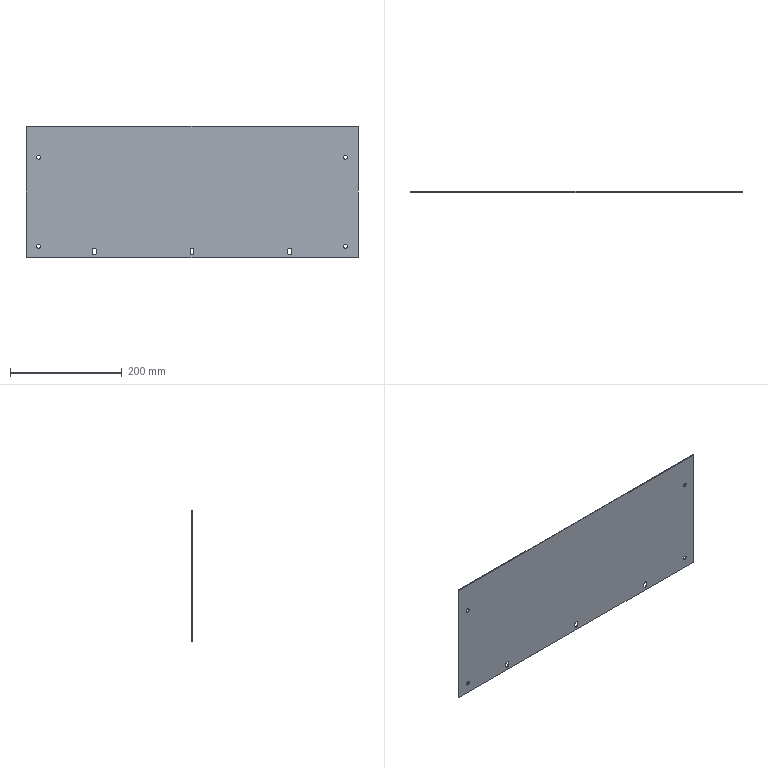Part | STEP file | PN_0023_cover plate_default_machined_ | 1 solid | 33 faces | box 595 x 1.5 x 235 mm | volume 209173 mm3 | cylinder 17 | plane 16 | commonest cylinder face diameters 7 x17